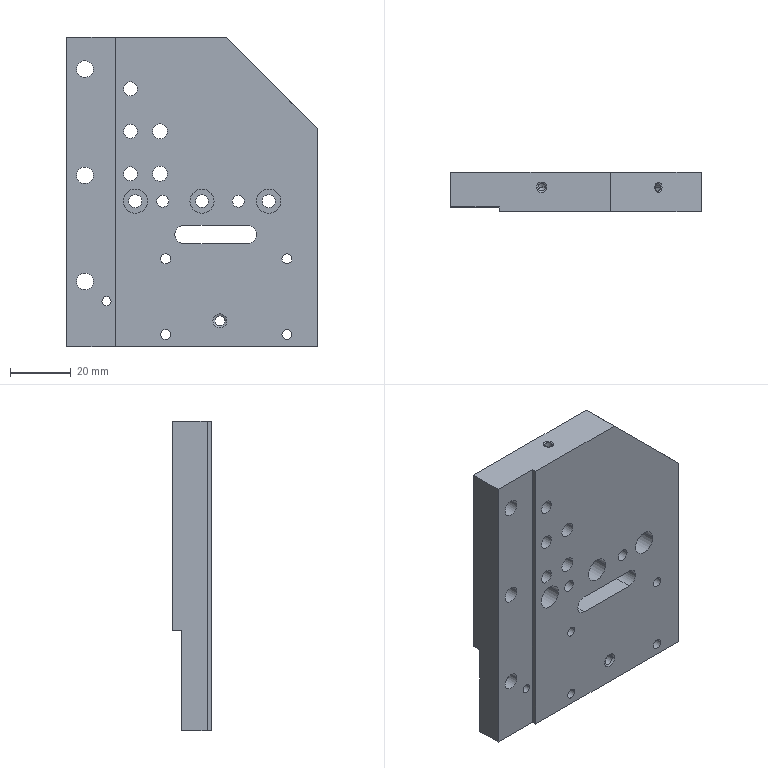Part | NX | 1 solid | 94 faces | box 82.6 x 13 x 102 mm | volume 85924 mm3 | cylinder 57 | plane 19 | cone 18 | commonest cylinder face diameters 3.3 x10 4.3 x6 4.6 x6 5.5 x6 8 x6 10 x6